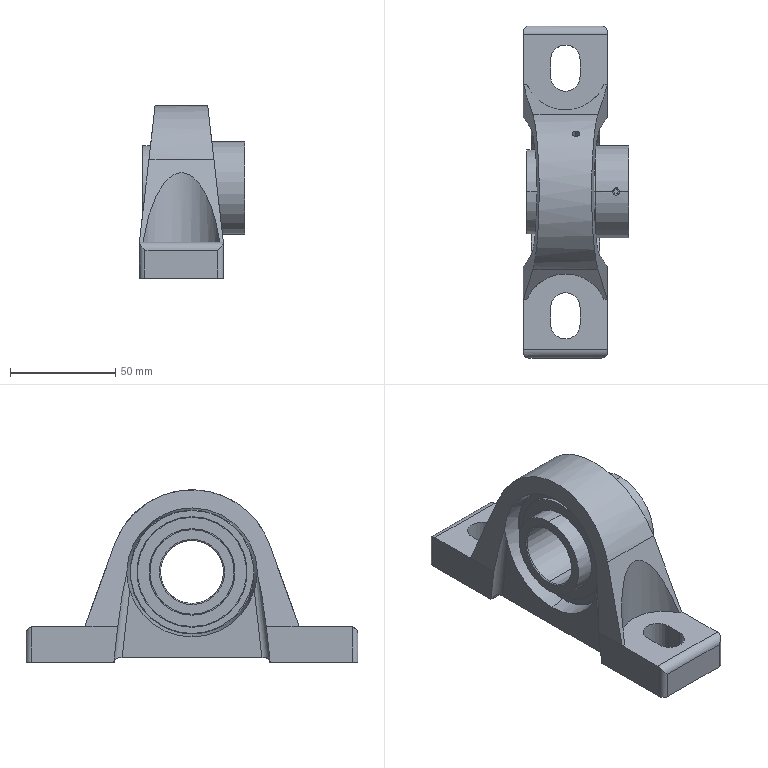Part | SolidWorks | 14 solids | 191 faces | box 50.1 x 158 x 82 mm | volume 190422 mm3 | cylinder 83 | plane 61 | spline 29 | cone 18 | commonest cylinder face diameters 40.2 x8 41.2 x8 52.667 x8 1 x4 4 x4 5.333 x4